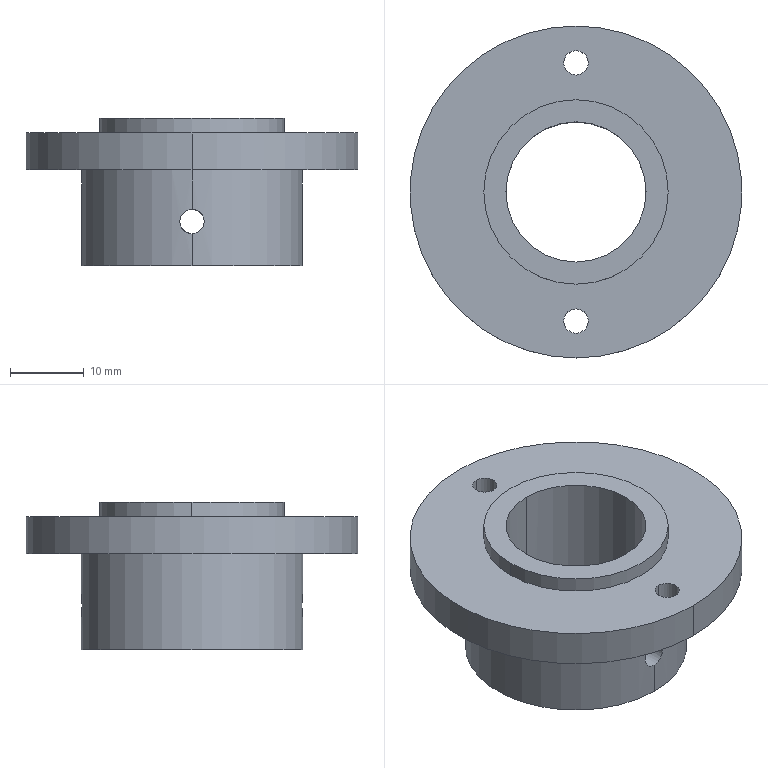Part | STEP file | 05-06 Alignment piece fixing seat | 1 solid | 20 faces | box 45 x 45 x 20 mm | volume 12273 mm3 | cylinder 16 | plane 4 | commonest cylinder face diameters 3.3 x8 19 x2 25 x2 30 x2 45 x2